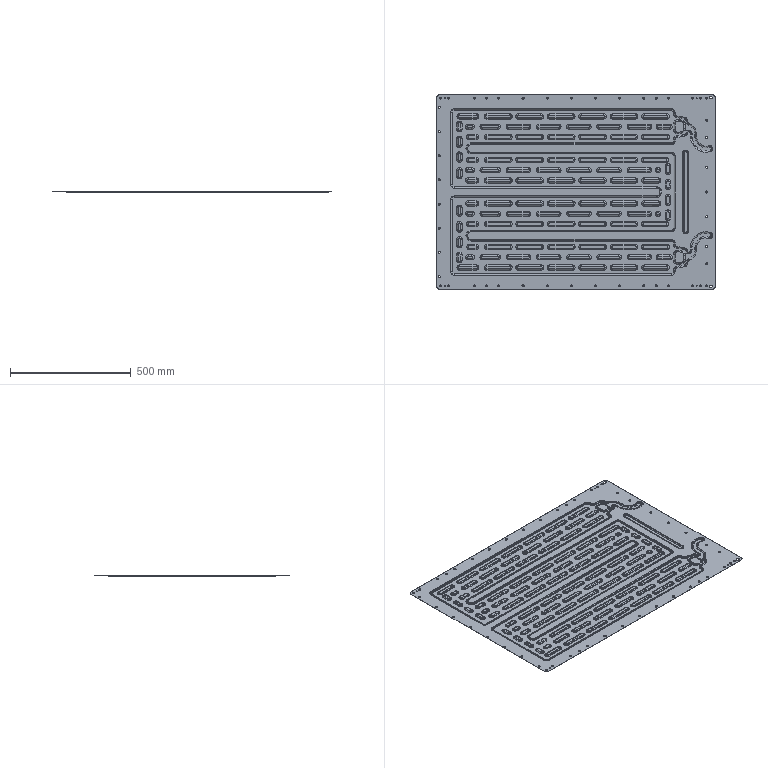Part | NX | features BREP 1 | 1 solid | 2588 faces | box 1150 x 803 x 4.5 mm | volume 1042892 mm3 | torus 1229 | cylinder 1048 | plane 218 | spline 93 | commonest cylinder face diameters 7 x352 5 x176 9 x176 8 x110 8.5 x94 6 x84